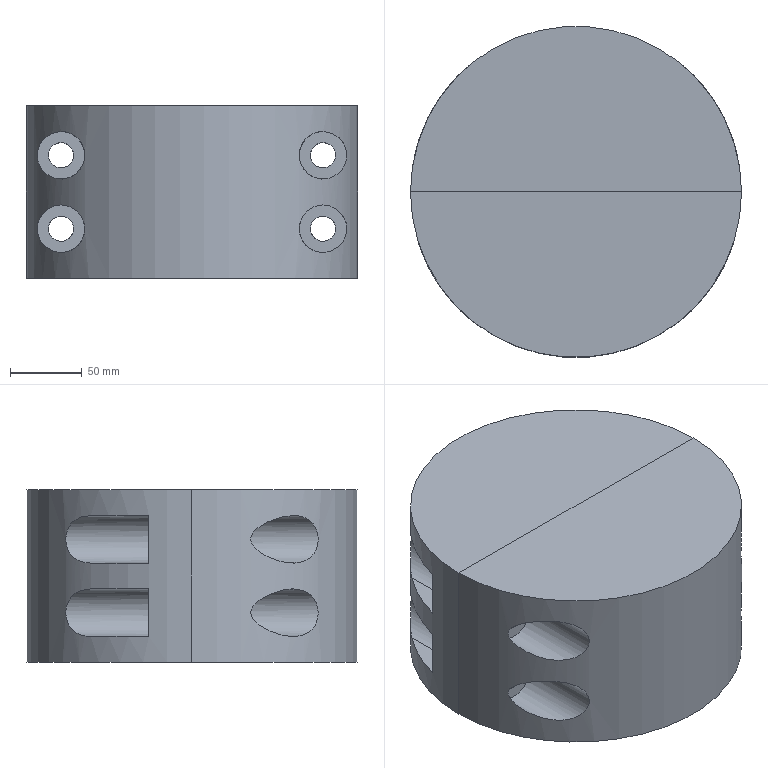NC program | NX | posted with a generic post | part box 230 x 230 x 120 mm
Lines 1 to 1053 of 7964:
N10 G17 G21 G94 G90
(ZLEVEL_PROFILE , TOOL : D25)
N12 T01 M6
N14 G54
N16 G17 G0 G90 X95.688 Y-23.744 S1000 M3
N18 G43 Z30. H1
N20 Z-25.213
N22 G94 G1 Z-26.713 F2000.
N24 X90.892 Y-22.
N26 G3 X88.43 Y-22.435 R2.5
N28 X88.435 Y-28.569 R4.002
N30 X90.897 Y-29. R2.5
N32 G1 X95.686 Y-27.251
N34 Z-25.213
N36 G0 X95.734 Y-27.074 Z-25.562
N38 G1 Z-27.062
N40 X91.032 Y-29.001
N42 G2 X88.555 Y-28.666 R2.5
N44 X87.363 Y-27.165 R4.006
N46 G1 X87.127 Y-26.5
N48 X87.011 Y-25.794
N50 X87.021 Y-25.087
N52 X87.16 Y-24.38
N54 G2 X88.549 Y-22.339 R4.001
N56 X91.026 Y-22. R2.5
N58 G1 X95.739 Y-23.924
N60 Z-25.562
N62 G0 X95.785 Y-24.06 Z-25.911
N64 G1 Z-27.411
N66 X91.125 Y-22.002
N68 G3 X88.639 Y-22.271 R2.5
N70 X88.642 Y-28.731 R4.
N72 X91.128 Y-28.998 R2.5
N74 G1 X95.782 Y-26.937
N76 Z-25.911
N78 G0 X95.824 Y-26.779 Z-26.26
N80 G1 Z-27.76
N82 X91.244 Y-28.991
N84 G2 X88.751 Y-28.808 R2.5
N86 X88.739 Y-22.2 R4.
N88 X91.232 Y-22.008 R2.5
N90 G1 X95.83 Y-24.209
N92 Z-26.26
N94 G0 X95.867 Y-24.371 Z-26.609
N96 G1 Z-28.109
N98 X91.349 Y-22.017
N100 G3 X88.852 Y-22.126 R2.5
N102 X88.859 Y-28.879 R4.
N104 X91.357 Y-28.982 R2.5
N106 G1 X95.86 Y-26.623
N108 Z-26.609
N110 G0 X95.892 Y-26.481 Z-26.958
N112 G1 Z-28.458
N114 X91.458 Y-28.97
N116 G2 X88.958 Y-28.94 R2.5
N118 X88.95 Y-22.065 R4.
N120 X91.449 Y-22.029 R2.5
N122 G1 X95.899 Y-24.512
N124 Z-26.958
N126 G0 X95.926 Y-24.654 Z-27.307
N128 G1 Z-28.807
N130 X91.55 Y-22.043
N132 G3 X89.05 Y-22.008 R2.5
N134 X89.054 Y-28.995 R4.
N136 X91.554 Y-28.956 R2.5
N138 G1 X95.921 Y-26.343
N140 Z-27.307
N142 G0 X95.941 Y-26.206 Z-27.656
N144 G1 Z-29.156
N146 X91.651 Y-28.939
N148 G2 X89.153 Y-29.048 R2.5
N150 X89.155 Y-21.951 R4.
N152 X91.653 Y-22.061 R2.5
N154 G1 X95.94 Y-24.797
N156 Z-27.656
N158 G0 X95.96 Y-24.929 Z-28.005
N160 G1 Z-29.505
N162 X91.743 Y-22.08
N164 G3 X89.249 Y-21.904 R2.5
N166 X89.248 Y-29.096 R4.
N168 X91.742 Y-28.921 R2.5
N170 G1 X95.961 Y-26.073
N172 Z-28.005
N174 G0 X95.973 Y-25.941 Z-28.354
N176 G1 Z-29.854
N178 X91.832 Y-28.9
N180 G2 X89.344 Y-29.141 R2.5
N182 X89.344 Y-21.859 R4.
N184 X91.833 Y-22.1 R2.5
N186 G1 X95.974 Y-25.06
N188 Z-28.354
N190 G0 X95.977 Y-25.192 Z-28.703
N192 G1 Z-30.203
N194 X91.927 Y-22.125
N196 G3 X89.446 Y-21.814 R2.5
N198 X89.437 Y-29.182 R4.
N200 X91.919 Y-28.877 R2.5
N202 G1 X95.984 Y-25.814
N204 Z-28.703
N206 G0 X95.992 Y-25.689 Z-29.052
N208 G1 Z-30.552
N210 X92.002 Y-28.854
N212 G2 X89.529 Y-29.22 R2.5
N214 X89.531 Y-21.78 R4.
N216 X92.004 Y-22.147 R2.5
N218 G1 X95.989 Y-25.312
N220 Z-29.052
N222 G0 X95.996 Y-25.433 Z-29.401
N224 G1 Z-30.901
N226 X92.083 Y-22.172
N228 G3 X89.619 Y-21.746 R2.5
N230 X89.628 Y-29.257 R4.
N232 X92.091 Y-28.826 R2.5
N234 G1 X95.988 Y-25.562
N236 Z-29.401
N238 G0 X100.275 Y-21.692 Z-29.75
N240 G1 Z-31.25
N242 X92.165 Y-28.8
N244 G2 X89.713 Y-29.287 R2.5
N246 X89.721 Y-21.71 R4.
N248 X92.172 Y-22.202 R2.5
N250 G1 X100.346 Y-29.395
N252 Z-29.75
N254 G0 X96.263 Y-25.501 Z-30.099
N256 G1 Z-31.599
N258 X92.248 Y-22.23
N260 G3 X89.808 Y-21.682 R2.5
N262 X89.807 Y-29.318 R4.
N264 X92.247 Y-28.77 R2.5
N266 G1 X96.263 Y-25.501
N268 Z-30.099
N270 G0 X96.456 Z-30.448
N272 G1 Z-31.948
N274 X92.316 Y-28.743
N276 G2 X89.888 Y-29.342 R2.5
N278 X89.897 Y-21.655 R4.
N280 X92.322 Y-22.259 R2.5
N282 G1 X96.456 Y-25.501
N284 Z-30.448
N286 G0 X96.668 Y-25.5 Z-30.797
N288 G1 Z-32.297
N290 X92.396 Y-22.29
N292 G3 X89.984 Y-21.631 R2.5
N294 X89.987 Y-29.37 R4.
N296 X92.398 Y-28.709 R2.5
N298 G1 X96.668 Y-25.5
N300 Z-30.797
N302 G0 X96.867 Z-31.146
N304 G1 Z-32.646
N306 X92.465 Y-28.679
N308 G2 X90.069 Y-29.39 R2.5
N310 X90.072 Y-21.609 R4.
N312 X92.468 Y-22.323 R2.5
N314 G1 X96.867 Y-25.5
N316 Z-31.146
N318 G0 X97.056 Y-25.501 Z-31.495
N320 G1 Z-32.995
N322 X92.516 Y-22.345
N324 G3 X90.131 Y-21.596 R2.5
N326 X90.145 Y-29.408 R4.
N328 X92.527 Y-28.649 R2.5
N330 G1 X97.056 Y-25.501
N332 Z-31.495
N334 G0 X97.285 Z-31.844
N336 G1 Z-33.344
N338 X92.588 Y-28.619
N340 G2 X90.222 Y-29.424 R2.5
N342 X90.222 Y-21.576 R4.
N344 X92.589 Y-22.382 R2.5
N346 G1 X97.285 Y-25.501
N348 Z-31.844
N350 G0 X97.55 Y-25.5 Z-32.193
N352 G1 Z-33.693
N354 X92.661 Y-22.419
N356 G3 X90.314 Y-21.559 R2.5
N358 X90.321 Y-29.442 R4.
N360 X92.666 Y-28.578 R2.5
N362 G1 X97.55 Y-25.5
N364 Z-32.193
N366 G0 X97.794 Z-32.543
N368 G1 Z-34.043
N370 X92.734 Y-28.54
N372 G2 X90.408 Y-29.456 R2.5
N374 X90.408 Y-21.544 R4.
N376 X92.734 Y-22.46 R2.5
N378 G1 X97.794 Y-25.5
N380 Z-32.543
N382 G0 X98.04 Y-25.502 Z-32.892
N384 G1 Z-34.392
N386 X92.794 Y-22.495
N388 G3 X90.486 Y-21.533 R2.5
N390 X90.486 Y-29.467 R4.
N392 X92.794 Y-28.506 R2.5
N394 G1 X98.04 Y-25.502
N396 Z-32.892
N398 G0 X98.284 Y-25.499 Z-33.241
N400 G1 Z-34.741
N402 X92.843 Y-28.475
N404 G2 X90.552 Y-29.475 R2.5
N406 X90.552 Y-21.525 R4.
N408 X92.843 Y-22.525 R2.5
N410 G1 X98.284 Y-25.499
N412 Z-33.241
N414 G0 X98.558 Z-33.59
N416 G1 Z-35.09
N418 X92.909 Y-22.566
N420 G3 X90.64 Y-21.516 R2.5
N422 X90.639 Y-29.484 R4.
N424 X92.908 Y-28.434 R2.5
N426 G1 X98.558 Y-25.499
N428 Z-33.59
N430 G0 X98.843 Z-33.939
N432 G1 Z-35.439
N434 X92.965 Y-28.397
N436 G2 X90.717 Y-29.49 R2.5
N438 X90.717 Y-21.51 R4.
N440 X92.965 Y-22.604 R2.5
N442 G1 X98.843 Y-25.499
N444 Z-33.939
N446 G0 X99.128 Y-25.5 Z-34.288
N448 G1 Z-35.788
N450 X93.018 Y-22.64
N452 G3 X90.791 Y-21.505 R2.5
N454 X90.791 Y-29.495 R4.
N456 X93.018 Y-28.36 R2.5
N458 G1 X99.128 Y-25.5
N460 Z-34.288
N462 G0 X99.43 Y-25.501 Z-34.637
N464 G1 Z-36.137
N466 X93.071 Y-28.321
N468 G2 X90.865 Y-29.498 R2.5
N470 X90.865 Y-21.502 R4.
N472 X93.071 Y-22.679 R2.5
N474 G1 X99.43 Y-25.501
N476 Z-34.637
N478 G0 X99.75 Y-25.499 Z-34.986
N480 G1 Z-36.486
N482 X93.134 Y-22.726
N484 G3 X90.955 Y-21.5 R2.5
N486 X90.955 Y-29.5 R4.
N488 X93.134 Y-28.274 R2.5
N490 G1 X99.75 Y-25.499
N492 Z-34.986
N494 G0 X100.049 Y-25.501 Z-35.335
N496 G1 Z-36.835
N498 X93.309 Y-28.25
N500 G2 X91.144 Y-29.5 R2.5
N502 G1 X91.
N504 G2 X87. Y-25.5 R4.
N506 X91. Y-21.5 R4.
N508 G1 X91.145
N510 G2 X93.31 Y-22.75 R2.5
N512 G1 X100.049 Y-25.501
N514 Z-35.335
N516 G0 X100.325 Z-35.684
N518 G1 Z-37.184
N520 X93.585 Y-22.75
N522 G3 X91.42 Y-21.5 R2.5
N524 G1 X91.
N526 G3 X87. Y-25.5 R4.
N528 X91. Y-29.5 R4.
N530 G1 X91.299
N532 G3 X93.464 Y-28.25 R2.5
N534 G1 X100.325 Y-25.501
N536 Z-35.684
N538 G0 X100.609 Y-25.5 Z-36.033
N540 G1 Z-37.533
N542 X93.851 Y-28.25
N544 G2 X91.686 Y-29.5 R2.5
N546 G1 X91.
N548 G2 X87. Y-25.5 R4.
N550 X91. Y-21.5 R4.
N552 G1 X91.51
N554 G2 X93.675 Y-22.75 R2.5
N556 G1 X100.609 Y-25.5
N558 Z-36.033
N560 G0 X100.884 Z-36.382
N562 G1 Z-37.882
N564 X94.135 Y-22.75
N566 G3 X91.97 Y-21.5 R2.5
N568 G1 X91.
N570 G3 X87. Y-25.5 R4.
N572 X91. Y-29.5 R4.
N574 G1 X91.98
N576 G3 X94.145 Y-28.25 R2.5
N578 G1 X100.884 Y-25.5
N580 Z-36.382
N582 G0 X101.16 Y-25.498 Z-36.731
N584 G1 Z-38.231
N586 X94.219 Y-28.25
N588 G2 X92.054 Y-29.5 R2.5
N590 G1 X91.
N592 G2 X87. Y-25.5 R4.
N594 X91. Y-21.5 R4.
N596 G1 X92.006
N598 G2 X94.171 Y-22.75 R2.5
N600 G1 X101.16 Y-25.498
N602 Z-36.731
N604 G0 X101.436 Y-25.499 Z-37.08
N606 G1 Z-38.58
N608 X94.697 Y-22.75
N610 G3 X92.532 Y-21.5 R2.5
N612 G1 X91.
N614 G3 X87. Y-25.5 R4.
N616 X91. Y-29.5 R4.
N618 G1 X92.53
N620 G3 X94.695 Y-28.25 R2.5
N622 G1 X101.436 Y-25.499
N624 Z-37.08
N626 G0 X101.714 Y-25.5 Z-37.429
N628 G1 Z-38.929
N630 X94.97 Y-28.25
N632 G2 X92.805 Y-29.5 R2.5
N634 G1 X91.
N636 G2 X87. Y-25.5 R4.
N638 X91. Y-21.5 R4.
N640 G1 X92.625
N642 G2 X94.79 Y-22.75 R2.5
N644 G1 X101.714 Y-25.5
N646 Z-37.429
N648 G0 X101.991 Z-37.778
N650 G1 Z-39.278
N652 X95.198 Y-22.75
N654 G3 X93.033 Y-21.5 R2.5
N656 G1 X91.
N658 G3 X87. Y-25.5 R4.
N660 X91. Y-29.5 R4.
N662 G1 X93.057
N664 G3 X95.222 Y-28.25 R2.5
N666 G1 X101.991 Y-25.5
N668 Z-37.778
N670 G0 X102.266 Y-25.499 Z-38.127
N672 G1 Z-39.627
N674 X95.522 Y-28.25
N676 G2 X93.357 Y-29.5 R2.5
N678 G1 X91.
N680 G2 X87. Y-25.5 R4.
N682 X91. Y-21.5 R4.
N684 G1 X93.362
N686 G2 X95.527 Y-22.75 R2.5
N688 G1 X102.266 Y-25.499
N690 Z-38.127
N692 G0 X102.544 Z-38.476
N694 G1 Z-39.976
N696 X95.804 Y-22.75
N698 G3 X93.639 Y-21.5 R2.5
N700 G1 X91.
N702 G3 X87. Y-25.5 R4.
N704 X91. Y-29.5 R4.
N706 G1 X93.506
N708 G3 X95.671 Y-28.25 R2.5
N710 G1 X102.544 Y-25.499
N712 Z-38.476
N714 G0 X102.82 Y-25.5 Z-38.825
N716 G1 Z-40.325
N718 X96.07 Y-28.25
N720 G2 X93.905 Y-29.5 R2.5
N722 G1 X91.
N724 G2 X87. Y-25.5 R4.
N726 X91. Y-21.5 R4.
N728 G1 X93.913
N730 G2 X96.078 Y-22.75 R2.5
N732 G1 X102.82 Y-25.5
N734 Z-38.825
N736 G0 X103.094 Y-25.501 Z-39.174
N738 G1 Z-40.674
N740 X96.296 Y-22.75
N742 G3 X94.131 Y-21.5 R2.5
N744 G1 X91.
N746 G3 X87. Y-25.5 R4.
N748 X91. Y-29.5 R4.
N750 G1 X94.004
N752 G3 X96.169 Y-28.25 R2.5
N754 G1 X103.094 Y-25.501
N756 Z-39.174
N758 G0 X103.373 Y-25.5 Z-39.523
N760 G1 Z-41.023
N762 X96.631 Y-28.25
N764 G2 X94.466 Y-29.5 R2.5
N766 G1 X91.
N768 G2 X87. Y-25.5 R4.
N770 X91. Y-21.5 R4.
N772 G1 X94.456
N774 G2 X96.621 Y-22.75 R2.5
N776 G1 X103.373 Y-25.5
N778 Z-39.523
N780 G0 X103.649 Z-39.872
N782 G1 Z-41.372
N784 X96.898 Y-22.75
N786 G3 X94.733 Y-21.5 R2.5
N788 G1 X91.
N790 G3 X87. Y-25.5 R4.
N792 X91. Y-29.5 R4.
N794 G1 X94.741
N796 G3 X96.906 Y-28.25 R2.5
N798 G1 X103.649 Y-25.5
N800 Z-39.872
N802 G0 X103.926 Z-40.221
N804 G1 Z-41.721
N806 X97.181 Y-28.25
N808 G2 X95.016 Y-29.5 R2.5
N810 G1 X91.
N812 G2 X87. Y-25.5 R4.
N814 X91. Y-21.5 R4.
N816 G1 X94.901
N818 G2 X97.066 Y-22.75 R2.5
N820 G1 X103.926 Y-25.5
N822 Z-40.221
N824 G0 X104.194 Y-25.501 Z-40.57
N826 G1 Z-42.07
N828 X97.457 Y-22.75
N830 G3 X95.292 Y-21.5 R2.5
N832 G1 X91.
N834 G3 X87. Y-25.5 R4.
N836 X91. Y-29.5 R4.
N838 G1 X95.106
N840 G3 X97.271 Y-28.25 R2.5
N842 G1 X104.194 Y-25.501
N844 Z-40.57
N846 G0 X104.453 Z-40.919
N848 G1 Z-42.419
N850 X97.618 Y-28.25
N852 G2 X95.453 Y-29.5 R2.5
N854 G1 X91.
N856 G2 X87. Y-25.5 R4.
N858 X91. Y-21.5 R4.
N860 G1 X95.553
N862 G2 X97.718 Y-22.75 R2.5
N864 G1 X104.453 Y-25.501
N866 Z-40.919
N868 G0 X104.718 Y-25.499 Z-41.268
N870 G1 Z-42.768
N872 X97.77 Y-22.75
N874 G3 X95.605 Y-21.5 R2.5
N876 G1 X91.
N878 G3 X87. Y-25.5 R4.
N880 X91. Y-29.5 R4.
N882 G1 X95.811
N884 G3 X97.976 Y-28.25 R2.5
N886 G1 X104.718 Y-25.499
N888 Z-41.268
N890 G0 X104.98 Y-25.5 Z-41.617
N892 G1 Z-43.117
N894 X98.232 Y-28.25
N896 G2 X96.067 Y-29.5 R2.5
N898 G1 X91.
N900 G2 X87. Y-25.5 R4.
N902 X91. Y-21.5 R4.
N904 G1 X96.071
N906 G2 X98.236 Y-22.75 R2.5
N908 G1 X104.98 Y-25.5
N910 Z-41.617
N912 G0 X105.239 Y-25.498 Z-41.966
N914 G1 Z-43.466
N916 X98.273 Y-22.75
N918 G3 X96.108 Y-21.5 R2.5
N920 G1 X91.
N922 G3 X87. Y-25.5 R4.
N924 X91. Y-29.5 R4.
N926 G1 X96.328
N928 G3 X98.493 Y-28.25 R2.5
N930 G1 X105.239 Y-25.498
N932 Z-41.966
N934 G0 X105.497 Y-25.5 Z-42.315
N936 G1 Z-43.815
N938 X98.737 Y-28.25
N940 G2 X96.572 Y-29.5 R2.5
N942 G1 X91.
N944 G2 X87. Y-25.5 R4.
N946 X91. Y-21.5 R4.
N948 G1 X96.551
N950 G2 X98.716 Y-22.75 R2.5
N952 G1 X105.497 Y-25.5
N954 Z-42.315
N956 G0 X105.762 Z-42.664
N958 G1 Z-44.164
N960 X99.014 Y-22.75
N962 G3 X96.849 Y-21.5 R2.5
N964 G1 X91.
N966 G3 X87. Y-25.5 R4.
N968 X91. Y-29.5 R4.
N970 G1 X96.763
N972 G3 X98.928 Y-28.25 R2.5
N974 G1 X105.762 Y-25.5
N976 Z-42.664
N978 G0 X106.018 Z-43.013
N980 G1 Z-44.513
N982 X99.172 Y-28.25
N984 G2 X97.006 Y-29.5 R2.5
N986 G1 X91.
N988 G2 X87. Y-25.5 R4.
N990 X91. Y-21.5 R4.
N992 G1 X97.108
N994 G2 X99.273 Y-22.75 R2.5
N996 G1 X106.018 Y-25.5
N998 Z-43.013
N1000 G0 X106.267 Z-43.362
N1002 G1 Z-44.862
N1004 X99.325 Y-22.75
N1006 G3 X97.16 Y-21.5 R2.5
N1008 G1 X91.
N1010 G3 X87. Y-25.5 R4.
N1012 X91. Y-29.5 R4.
N1014 G1 X97.257
N1016 G3 X99.422 Y-28.25 R2.5
N1018 G1 X106.267 Y-25.5
N1020 Z-43.362
N1022 G0 X106.507 Y-25.501 Z-43.711
N1024 G1 Z-45.211
N1026 X99.761 Y-28.25
N1028 G2 X97.596 Y-29.5 R2.5
N1030 G1 X91.
N1032 G2 X87. Y-25.5 R4.
N1034 X91. Y-21.5 R4.
N1036 G1 X97.595
N1038 G2 X99.761 Y-22.75 R2.5
N1040 G1 X106.507 Y-25.501
N1042 Z-43.711
N1044 G0 X106.761 Y-25.499 Z-44.06
N1046 G1 Z-45.56
N1048 X99.926 Y-22.75
N1050 G3 X97.761 Y-21.5 R2.5
N1052 G1 X91.
N1054 G3 X87. Y-25.5 R4.
N1056 X91. Y-29.5 R4.
N1058 G1 X97.847
N1060 G3 X100.012 Y-28.25 R2.5
N1062 G1 X106.761 Y-25.499
N1064 Z-44.06
N1066 G0 X107.008 Z-44.409
N1068 G1 Z-45.909
N1070 X100.086 Y-28.25
N1072 G2 X97.921 Y-29.5 R2.5
N1074 G1 X91.
N1076 G2 X87. Y-25.5 R4.
N1078 X91. Y-21.5 R4.
N1080 G1 X98.099
N1082 G2 X100.264 Y-22.75 R2.5
N1084 G1 X107.008 Y-25.499
N1086 Z-44.409
N1088 G0 X107.25 Y-25.501 Z-44.758
N1090 G1 Z-46.258
N1092 X100.477 Y-22.75
N1094 G3 X98.312 Y-21.5 R2.5
N1096 G1 X91.
N1098 G3 X87. Y-25.5 R4.
N1100 X91. Y-29.5 R4.
N1102 G1 X98.243
N1104 G3 X100.408 Y-28.25 R2.5
N1106 G1 X107.25 Y-25.501
N1108 Z-44.758
N1110 G0 X107.496 Z-45.107
N1112 G1 Z-46.607
N1114 X100.757 Y-28.25
N1116 G2 X98.592 Y-29.5 R2.5
N1118 G1 X91.
N1120 G2 X87. Y-25.5 R4.
N1122 X91. Y-21.5 R4.
N1124 G1 X98.592
N1126 G2 X100.757 Y-22.75 R2.5
N1128 G1 X107.496 Y-25.501
N1130 Z-45.107
N1132 G0 X107.744 Y-25.5 Z-45.456
N1134 G1 Z-46.956
N1136 X100.999 Y-22.75
N1138 G3 X98.834 Y-21.5 R2.5
N1140 G1 X91.
N1142 G3 X87. Y-25.5 R4.
N1144 X91. Y-29.5 R4.
N1146 G1 X98.834
N1148 G3 X100.999 Y-28.25 R2.5
N1150 G1 X107.744 Y-25.5
N1152 Z-45.456
N1154 G0 X107.984 Y-25.499 Z-45.805
N1156 G1 Z-47.305
N1158 X101.069 Y-28.25
N1160 G2 X98.904 Y-29.5 R2.5
N1162 G1 X91.
N1164 G2 X87. Y-25.5 R4.
N1166 X91. Y-21.5 R4.
N1168 G1 X98.99
N1170 G2 X101.155 Y-22.75 R2.5
N1172 G1 X107.984 Y-25.499
N1174 Z-45.805
N1176 G0 X108.211 Y-25.5 Z-46.154
N1178 G1 Z-47.654
N1180 X101.471 Y-22.75
N1182 G3 X99.306 Y-21.5 R2.5
N1184 G1 X91.
N1186 G3 X87. Y-25.5 R4.
N1188 X91. Y-29.5 R4.
N1190 G1 X99.306
N1192 G3 X101.471 Y-28.25 R2.5
N1194 G1 X108.211 Y-25.5
N1196 Z-46.154
N1198 G0 X108.449 Y-25.499 Z-46.503
N1200 G1 Z-48.003
N1202 X101.702 Y-28.25
N1204 G2 X99.537 Y-29.5 R2.5
N1206 G1 X91.
N1208 G2 X87. Y-25.5 R4.
N1210 X91. Y-21.5 R4.
N1212 G1 X99.537
N1214 G2 X101.702 Y-22.75 R2.5
N1216 G1 X108.449 Y-25.499
N1218 Z-46.503
N1220 G0 X108.683 Y-25.5 Z-46.852
N1222 G1 Z-48.352
N1224 X101.862 Y-22.75
N1226 G3 X99.697 Y-21.5 R2.5
N1228 G1 X91.
N1230 G3 X87. Y-25.5 R4.
N1232 X91. Y-29.5 R4.
N1234 G1 X99.768
N1236 G3 X101.933 Y-28.25 R2.5
N1238 G1 X108.683 Y-25.5
N1240 Z-46.852
N1242 G0 X108.913 Y-25.502 Z-47.202
N1244 G1 Z-48.702
N1246 X102.176 Y-28.25
N1248 G2 X100.011 Y-29.5 R2.5
N1250 G1 X91.
N1252 G2 X87. Y-25.5 R4.
N1254 X91. Y-21.5 R4.
N1256 G1 X100.009
N1258 G2 X102.174 Y-22.75 R2.5
N1260 G1 X108.913 Y-25.502
N1262 Z-47.202
N1264 G0 X109.143 Y-25.5 Z-47.551
N1266 G1 Z-49.051
N1268 X102.405 Y-22.75
N1270 G3 X100.24 Y-21.5 R2.5
N1272 G1 X91.
N1274 G3 X87. Y-25.5 R4.
N1276 X91. Y-29.5 R4.
N1278 G1 X100.232
N1280 G3 X102.397 Y-28.25 R2.5
N1282 G1 X109.143 Y-25.5
N1284 Z-47.551
N1286 G0 X109.382 Y-25.499 Z-47.9
N1288 G1 Z-49.4
N1290 X102.639 Y-28.25
N1292 G2 X100.474 Y-29.5 R2.5
N1294 G1 X91.
N1296 G2 X87. Y-25.5 R4.
N1298 X91. Y-21.5 R4.
N1300 G1 X100.413
N1302 G2 X102.578 Y-22.75 R2.5
N1304 G1 X109.382 Y-25.499
N1306 Z-47.9
N1308 G0 X109.609 Z-48.249
N1310 G1 Z-49.749
N1312 X102.772 Y-22.75
N1314 G3 X100.607 Y-21.5 R2.5
N1316 G1 X91.
N1318 G3 X87. Y-25.5 R4.
N1320 X91. Y-29.5 R4.
N1322 G1 X100.707
N1324 G3 X102.872 Y-28.25 R2.5
N1326 G1 X109.609 Y-25.499
N1328 Z-48.249
N1330 G0 X109.831 Z-48.598
N1332 G1 Z-50.098
N1334 X103.08 Y-28.25
N1336 G2 X100.915 Y-29.5 R2.5
N1338 G1 X91.
N1340 G2 X87. Y-25.5 R4.
N1342 X91. Y-21.5 R4.
N1344 G1 X100.92
N1346 G2 X103.085 Y-22.75 R2.5
N1348 G1 X109.831 Y-25.499
N1350 Z-48.598
N1352 G0 X110.051 Z-48.947
N1354 G1 Z-50.447
N1356 X103.244 Y-22.75
N1358 G3 X101.079 Y-21.5 R2.5
N1360 G1 X91.
N1362 G3 X87. Y-25.5 R4.
N1364 X91. Y-29.5 R4.
N1366 G1 X101.141
N1368 G3 X103.307 Y-28.25 R2.5
N1370 G1 X110.051 Y-25.499
N1372 Z-48.947
N1374 G0 X110.273 Z-49.296
N1376 G1 Z-50.796
N1378 X103.432 Y-28.25
N1380 G2 X101.267 Y-29.5 R2.5
N1382 G1 X91.
N1384 G2 X87. Y-25.5 R4.
N1386 X91. Y-21.5 R4.
N1388 G1 X101.308
N1390 G2 X103.473 Y-22.75 R2.5
N1392 G1 X110.273 Y-25.499
N1394 Z-49.296
N1396 G0 X110.493 Z-49.645
N1398 G1 Z-51.145
N1400 X103.697 Y-22.75
N1402 G3 X101.532 Y-21.5 R2.5
N1404 G1 X91.
N1406 G3 X87. Y-25.5 R4.
N1408 X91. Y-29.5 R4.
N1410 G1 X101.524
N1412 G3 X103.689 Y-28.25 R2.5
N1414 G1 X110.493 Y-25.499
N1416 Z-49.645
N1418 G0 X110.711 Z-49.994
N1420 G1 Z-51.494
N1422 X103.941 Y-28.25
N1424 G2 X101.776 Y-29.5 R2.5
N1426 G1 X91.
N1428 G2 X87. Y-25.5 R4.
N1430 X91. Y-21.5 R4.
N1432 G1 X101.707
N1434 G2 X103.872 Y-22.75 R2.5
N1436 G1 X110.711 Y-25.499
N1438 Z-49.994
N1440 G0 X110.931 Z-50.343
N1442 G1 Z-51.843
N1444 X104.148 Y-22.75
N1446 G3 X101.983 Y-21.5 R2.5
N1448 G1 X91.
N1450 G3 X87. Y-25.5 R4.
N1452 X91. Y-29.5 R4.
N1454 G1 X102.001
N1456 G3 X104.166 Y-28.25 R2.5
N1458 G1 X110.931 Y-25.499
N1460 Z-50.343
N1462 G0 X111.152 Y-25.5 Z-50.692
N1464 G1 Z-52.192
N1466 X104.41 Y-28.25
N1468 G2 X102.245 Y-29.5 R2.5
N1470 G1 X91.
N1472 G2 X87. Y-25.5 R4.
N1474 X91. Y-21.5 R4.
N1476 G1 X102.234
N1478 G2 X104.399 Y-22.75 R2.5
N1480 G1 X111.152 Y-25.5
N1482 Z-50.692
N1484 G0 X111.364 Y-25.499 Z-51.041
N1486 G1 Z-52.541
N1488 X104.598 Y-22.75
N1490 G3 X102.433 Y-21.5 R2.5
N1492 G1 X91.
N1494 G3 X87. Y-25.5 R4.
N1496 X91. Y-29.5 R4.
N1498 G1 X102.45
N1500 G3 X104.615 Y-28.25 R2.5
N1502 G1 X111.364 Y-25.499
N1504 Z-51.041
N1506 G0 X111.571 Z-51.39
N1508 G1 Z-52.89
N1510 X104.756 Y-28.25
N1512 G2 X102.591 Y-29.5 R2.5
N1514 G1 X91.
N1516 G2 X87. Y-25.5 R4.
N1518 X91. Y-21.5 R4.
N1520 G1 X102.644
N1522 G2 X104.809 Y-22.75 R2.5
N1524 G1 X111.571 Y-25.499
N1526 Z-51.39
N1528 G0 X111.78 Z-51.739
N1530 G1 Z-53.239
N1532 X105.019 Y-22.75
N1534 G3 X102.854 Y-21.5 R2.5
N1536 G1 X91.
N1538 G3 X87. Y-25.5 R4.
N1540 X91. Y-29.5 R4.
N1542 G1 X102.835
N1544 G3 X105. Y-28.25 R2.5
N1546 G1 X111.78 Y-25.499
N1548 Z-51.739
N1550 G0 X111.986 Z-52.088
N1552 G1 Z-53.588
N1554 X105.243 Y-28.25
N1556 G2 X103.078 Y-29.5 R2.5
N1558 G1 X91.
N1560 G2 X87. Y-25.5 R4.
N1562 X91. Y-21.5 R4.
N1564 G1 X103.08
N1566 G2 X105.245 Y-22.75 R2.5
N1568 G1 X111.986 Y-25.499
N1570 Z-52.088
N1572 G0 X112.196 Z-52.437
N1574 G1 Z-53.937
N1576 X105.398 Y-22.75
N1578 G3 X103.233 Y-21.5 R2.5
N1580 G1 X91.
N1582 G3 X87. Y-25.5 R4.
N1584 X91. Y-29.5 R4.
N1586 G1 X103.257
N1588 G3 X105.422 Y-28.25 R2.5
N1590 G1 X112.196 Y-25.499
N1592 Z-52.437
N1594 G0 X112.401 Z-52.786
N1596 G1 Z-54.286
N1598 X105.663 Y-28.25
N1600 G2 X103.498 Y-29.5 R2.5
N1602 G1 X91.
N1604 G2 X87. Y-25.5 R4.
N1606 X91. Y-21.5 R4.
N1608 G1 X103.358
N1610 G2 X105.523 Y-22.75 R2.5
N1612 G1 X112.401 Y-25.499
N1614 Z-52.786
N1616 G0 X112.61 Z-53.135
N1618 G1 Z-54.635
N1620 X105.799 Y-22.75
N1622 G3 X103.634 Y-21.5 R2.5
N1624 G1 X91.
N1626 G3 X87. Y-25.5 R4.
N1628 X91. Y-29.5 R4.
N1630 G1 X103.626
N1632 G3 X105.791 Y-28.25 R2.5
N1634 G1 X112.61 Y-25.499
N1636 Z-53.135
N1638 G0 X112.817 Y-25.5 Z-53.484
N1640 G1 Z-54.984
N1642 X106.047 Y-28.25
N1644 G2 X103.882 Y-29.5 R2.5
N1646 G1 X91.
N1648 G2 X87. Y-25.5 R4.
N1650 X91. Y-21.5 R4.
N1652 G1 X103.816
N1654 G2 X105.981 Y-22.75 R2.5
N1656 G1 X112.817 Y-25.5
N1658 Z-53.484
N1660 G0 X113.014 Y-25.499 Z-53.833
N1662 G1 Z-55.333
N1664 X106.125 Y-22.75
N1666 G3 X103.96 Y-21.5 R2.5
N1668 G1 X91.
N1670 G3 X87. Y-25.5 R4.
N1672 X91. Y-29.5 R4.
N1674 G1 X104.106
N1676 G3 X106.271 Y-28.25 R2.5
N1678 G1 X113.014 Y-25.499
N1680 Z-53.833
N1682 G0 X113.209 Z-54.182
N1684 G1 Z-55.682
N1686 X106.386 Y-28.25
N1688 G2 X104.221 Y-29.5 R2.5
N1690 G1 X91.
N1692 G2 X87. Y-25.5 R4.
N1694 X91. Y-21.5 R4.
N1696 G1 X104.243
N1698 G2 X106.408 Y-22.75 R2.5
N1700 G1 X113.209 Y-25.499
N1702 Z-54.182
N1704 G0 X113.405 Z-54.531
N1706 G1 Z-56.031
N1708 X106.653 Y-22.75
N1710 G3 X104.488 Y-21.5 R2.5
N1712 G1 X91.
N1714 G3 X87. Y-25.5 R4.
N1716 X91. Y-29.5 R4.
N1718 G1 X104.501
N1720 G3 X106.666 Y-28.25 R2.5
N1722 G1 X113.405 Y-25.499
N1724 Z-54.531
N1726 G0 X113.601 Y-25.5 Z-54.88
N1728 G1 Z-56.38
N1730 X106.698 Y-28.25
N1732 G2 X104.533 Y-29.5 R2.5
N1734 G1 X91.
N1736 G2 X87. Y-25.5 R4.
N1738 X91. Y-21.5 R4.
N1740 G1 X104.646
N1742 G2 X106.811 Y-22.75 R2.5
N1744 G1 X113.601 Y-25.5
N1746 Z-54.88
N1748 G0 X113.796 Z-55.229
N1750 G1 Z-56.729
N1752 X107.031 Y-22.75
N1754 G3 X104.866 Y-21.5 R2.5
N1756 G1 X91.
N1758 G3 X87. Y-25.5 R4.
N1760 X91. Y-29.5 R4.
N1762 G1 X104.835
N1764 G3 X107. Y-28.25 R2.5
N1766 G1 X113.796 Y-25.5
N1768 Z-55.229
N1770 G0 X113.991 Z-55.578
N1772 G1 Z-57.078
N1774 X107.234 Y-28.25
N1776 G2 X105.069 Y-29.5 R2.5
N1778 G1 X91.
N1780 G2 X87. Y-25.5 R4.
N1782 X91. Y-21.5 R4.
N1784 G1 X105.076
N1786 G2 X107.241 Y-22.75 R2.5
N1788 G1 X113.991 Y-25.5
N1790 Z-55.578
N1792 G0 X114.187 Z-55.927
N1794 G1 Z-57.427
N1796 X107.398 Y-22.75
N1798 G3 X105.233 Y-21.5 R2.5
N1800 G1 X91.
N1802 G3 X87. Y-25.5 R4.
N1804 X91. Y-29.5 R4.
N1806 G1 X105.282
N1808 G3 X107.447 Y-28.25 R2.5
N1810 G1 X114.187 Y-25.5
N1812 Z-55.927
N1814 G0 X114.384 Y-25.502 Z-56.276
N1816 G1 Z-57.776
N1818 X107.592 Y-28.25
N1820 G2 X105.427 Y-29.5 R2.5
N1822 G1 X91.
N1824 G2 X87. Y-25.5 R4.
N1826 X91. Y-21.5 R4.
N1828 G1 X105.355
N1830 G2 X107.52 Y-22.75 R2.5
N1832 G1 X114.384 Y-25.502
N1834 Z-56.276
N1836 G0 X114.563 Y-25.499 Z-56.625
N1838 G1 Z-58.125
N1840 X107.679 Y-22.75
N1842 G3 X105.514 Y-21.5 R2.5
N1844 G1 X91.
N1846 G3 X87. Y-25.5 R4.
N1848 X91. Y-29.5 R4.
N1850 G1 X105.658
N1852 G3 X107.823 Y-28.25 R2.5
N1854 G1 X114.563 Y-25.499
N1856 Z-56.625
N1858 G0 X114.749 Y-25.5 Z-56.974
N1860 G1 Z-58.474
N1862 X107.937 Y-28.25
N1864 G2 X105.772 Y-29.5 R2.5
N1866 G1 X91.
N1868 G2 X87. Y-25.5 R4.
N1870 X91. Y-21.5 R4.
N1872 G1 X105.692
N1874 G2 X107.857 Y-22.75 R2.5
N1876 G1 X114.749 Y-25.5
N1878 Z-56.974
N1880 G0 X114.932 Y-25.499 Z-57.323
N1882 G1 Z-58.823
N1884 X108.187 Y-22.75
N1886 G3 X106.022 Y-21.5 R2.5
N1888 G1 X91.
N1890 G3 X87. Y-25.5 R4.
N1892 X91. Y-29.5 R4.
N1894 G1 X105.916
N1896 G3 X108.081 Y-28.25 R2.5
N1898 G1 X114.932 Y-25.499
N1900 Z-57.323
N1902 G0 X115.117 Y-25.5 Z-57.672
N1904 G1 Z-59.172
N1906 X108.238 Y-28.25
N1908 G2 X106.073 Y-29.5 R2.5
N1910 G1 X91.
N1912 G2 X87. Y-25.5 R4.
N1914 X91. Y-21.5 R4.
N1916 G1 X106.131
N1918 G2 X108.296 Y-22.75 R2.5
N1920 G1 X115.117 Y-25.5
N1922 Z-57.672
N1924 G0 X115.3 Y-25.499 Z-58.021
N1926 G1 Z-59.521
N1928 X108.531 Y-22.75
N1930 G3 X106.366 Y-21.5 R2.5
N1932 G1 X91.
N1934 G3 X87. Y-25.5 R4.
N1936 X91. Y-29.5 R4.
N1938 G1 X106.349
N1940 G3 X108.515 Y-28.25 R2.5
N1942 G1 X115.3 Y-25.499
N1944 Z-58.021
N1946 G0 X115.483 Z-58.37
N1948 G1 Z-59.87
N1950 X108.743 Y-28.25
N1952 G2 X106.578 Y-29.5 R2.5
N1954 G1 X91.
N1956 G2 X87. Y-25.5 R4.
N1958 X91. Y-21.5 R4.
N1960 G1 X106.578
N1962 G2 X108.743 Y-22.75 R2.5
N1964 G1 X115.483 Y-25.499
N1966 Z-58.37
N1968 G0 X115.666 Y-25.5 Z-58.719
N1970 G1 Z-60.219
N1972 X108.921 Y-22.75
N1974 G3 X106.755 Y-21.5 R2.5
N1976 G1 X91.
N1978 G3 X87. Y-25.5 R4.
N1980 X91. Y-29.5 R4.
N1982 G1 X106.707
N1984 G3 X108.872 Y-28.25 R2.5
N1986 G1 X115.666 Y-25.5
N1988 Z-58.719
N1990 G0 X115.848 Z-59.068
N1992 G1 Z-60.568
N1994 X109.104 Y-28.25
N1996 G2 X106.939 Y-29.5 R2.5
N1998 G1 X91.
N2000 G2 X87. Y-25.5 R4.
N2002 X91. Y-21.5 R4.
N2004 G1 X106.865
N2006 G2 X109.03 Y-22.75 R2.5
N2008 G1 X115.848 Y-25.5
N2010 Z-59.068
N2012 G0 X116.021 Z-59.417
N2014 G1 Z-60.917
N2016 X109.221 Y-22.75
N2018 G3 X107.056 Y-21.5 R2.5
N2020 G1 X91.
N2022 G3 X87. Y-25.5 R4.
N2024 X91. Y-29.5 R4.
N2026 G1 X107.041
N2028 G3 X109.206 Y-28.25 R2.5
N2030 G1 X116.021 Y-25.5
N2032 Z-59.417
N2034 G0 X116.193 Y-25.499 Z-59.766
N2036 G1 Z-61.266
N2038 X109.446 Y-28.25
N2040 G2 X107.281 Y-29.5 R2.5
N2042 G1 X91.
N2044 G2 X87. Y-25.5 R4.
N2046 X91. Y-21.5 R4.
N2048 G1 X107.281
N2050 G2 X109.446 Y-22.75 R2.5
N2052 G1 X116.193 Y-25.499
N2054 Z-59.766
N2056 G0 X116.366 Z-60.115
N2058 G1 Z-61.615
N2060 X109.521 Y-22.75
N2062 G3 X107.356 Y-21.5 R2.5
N2064 G1 X91.
N2066 G3 X87. Y-25.5 R4.
N2068 X91. Y-29.5 R4.
N2070 G1 X107.436
N2072 G3 X109.601 Y-28.25 R2.5
N2074 G1 X116.366 Y-25.499
N2076 Z-60.115
N2078 G0 X116.537 Y-25.5 Z-60.464
N2080 G1 Z-61.964
N2082 X109.703 Y-28.25
N2084 G2 X107.538 Y-29.5 R2.5
N2086 G1 X91.
N2088 G2 X87. Y-25.5 R4.
N2090 X91. Y-21.5 R4.
N2092 G1 X107.505
N2094 G2 X109.671 Y-22.75 R2.5
N2096 G1 X116.537 Y-25.5
N2098 Z-60.464
N2100 G0 X116.71 Y-25.499 Z-60.813
N2102 G1 Z-62.313
N2104 X109.936 Y-22.75